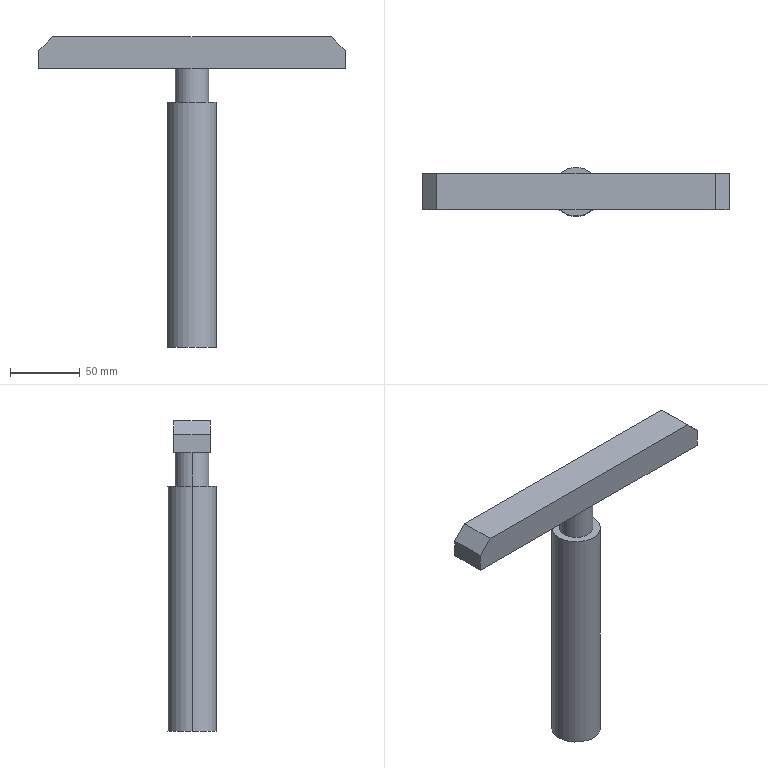Part | SolidWorks | features ICE 2, Chamfer 1, Extrusion 1 | 1 solid | 14 faces | box 220 x 35 x 223 mm | volume 309149 mm3 | plane 10 | cylinder 4 | commonest cylinder face diameters 24 x2 35 x2
STEP:
#1=CARTESIAN_POINT('',(12.,0.,176.));
#2=VERTEX_POINT('',#1);
#3=CARTESIAN_POINT('',(-12.,0.,176.));
#4=VERTEX_POINT('',#3);
#5=CARTESIAN_POINT('',(0.,0.,176.));
#6=DIRECTION('',(0.,0.,1.));
#7=DIRECTION('',(1.,0.,0.));
#8=AXIS2_PLACEMENT_3D('',#5,#6,#7);
#9=CIRCLE('',#8,12.);
#10=EDGE_CURVE('',#2,#4,#9,.T.);
#11=ORIENTED_EDGE('',*,*,#10,.T.);
#12=CARTESIAN_POINT('',(-12.,0.,200.));
#13=VERTEX_POINT('',#12);
#14=CARTESIAN_POINT('',(-12.,0.,176.));
#15=DIRECTION('',(0.,0.,1.));
#16=VECTOR('',#15,1000.);
#17=LINE('',#14,#16);
#18=EDGE_CURVE('',#4,#13,#17,.T.);
#19=ORIENTED_EDGE('',*,*,#18,.T.);
#20=CARTESIAN_POINT('',(12.,0.,200.));
#21=VERTEX_POINT('',#20);
#22=CARTESIAN_POINT('',(0.,0.,200.));
#23=DIRECTION('',(0.,0.,1.));
#24=DIRECTION('',(1.,0.,0.));
#25=AXIS2_PLACEMENT_3D('',#22,#23,#24);
#26=CIRCLE('',#25,12.);
#27=EDGE_CURVE('',#21,#13,#26,.T.);
#28=ORIENTED_EDGE('',*,*,#27,.F.);
#29=CARTESIAN_POINT('',(12.,0.,176.));
#30=DIRECTION('',(0.,0.,1.));
#31=VECTOR('',#30,1000.);
#32=LINE('',#29,#31);
#33=EDGE_CURVE('',#2,#21,#32,.T.);
#34=ORIENTED_EDGE('',*,*,#33,.F.);
#35=EDGE_LOOP('',(#11,#19,#28,#34));
#36=FACE_OUTER_BOUND('',#35,.T.);
#37=CARTESIAN_POINT('',(0.,0.,176.));
#38=DIRECTION('',(0.,0.,1.));
#39=DIRECTION('',(1.,0.,0.));
#40=AXIS2_PLACEMENT_3D('',#37,#38,#39);
#41=CYLINDRICAL_SURFACE('',#40,12.);
#42=ADVANCED_FACE('',(#36),#41,.T.);
#43=CARTESIAN_POINT('',(17.5,0.,176.));
#44=VERTEX_POINT('',#43);
#45=CARTESIAN_POINT('',(-17.5,0.,176.));
#46=VERTEX_POINT('',#45);
#47=CARTESIAN_POINT('',(0.,0.,176.));
#48=DIRECTION('',(0.,0.,1.));
#49=DIRECTION('',(1.,0.,0.));
#50=AXIS2_PLACEMENT_3D('',#47,#48,#49);
#51=CIRCLE('',#50,17.5);
#52=EDGE_CURVE('',#44,#46,#51,.T.);
#53=ORIENTED_EDGE('',*,*,#52,.F.);
#54=CARTESIAN_POINT('',(17.5,0.,0.));
#55=VERTEX_POINT('',#54);
#56=CARTESIAN_POINT('',(17.5,0.,200.));
#57=DIRECTION('',(0.,0.,-1.));
#58=VECTOR('',#57,1000.);
#59=LINE('',#56,#58);
#60=EDGE_CURVE('',#44,#55,#59,.T.);
#61=ORIENTED_EDGE('',*,*,#60,.T.);
#62=CARTESIAN_POINT('',(-17.5,0.,0.));
#63=VERTEX_POINT('',#62);
#64=CARTESIAN_POINT('',(0.,0.,0.));
#65=DIRECTION('',(0.,0.,1.));
#66=DIRECTION('',(1.,0.,0.));
#67=AXIS2_PLACEMENT_3D('',#64,#65,#66);
#68=CIRCLE('',#67,17.5);
#69=EDGE_CURVE('',#55,#63,#68,.T.);
#70=ORIENTED_EDGE('',*,*,#69,.T.);
#71=CARTESIAN_POINT('',(-17.5,0.,200.));
#72=DIRECTION('',(0.,0.,-1.));
#73=VECTOR('',#72,1000.);
#74=LINE('',#71,#73);
#75=EDGE_CURVE('',#46,#63,#74,.T.);
#76=ORIENTED_EDGE('',*,*,#75,.F.);
#77=EDGE_LOOP('',(#53,#61,#70,#76));
#78=FACE_OUTER_BOUND('',#77,.T.);
#79=CARTESIAN_POINT('',(0.,0.,200.));
#80=DIRECTION('',(0.,0.,-1.));
#81=DIRECTION('',(-1.,0.,0.));
#82=AXIS2_PLACEMENT_3D('',#79,#80,#81);
#83=CYLINDRICAL_SURFACE('',#82,17.5);
#84=ADVANCED_FACE('',(#78),#83,.T.);
#85=ORIENTED_EDGE('',*,*,#60,.F.);
#86=CARTESIAN_POINT('',(0.,0.,176.));
#87=DIRECTION('',(0.,0.,1.));
#88=DIRECTION('',(1.,0.,0.));
#89=AXIS2_PLACEMENT_3D('',#86,#87,#88);
#90=CIRCLE('',#89,17.5);
#91=EDGE_CURVE('',#46,#44,#90,.T.);
#92=ORIENTED_EDGE('',*,*,#91,.F.);
#93=ORIENTED_EDGE('',*,*,#75,.T.);
#94=CARTESIAN_POINT('',(0.,0.,0.));
#95=DIRECTION('',(0.,0.,1.));
#96=DIRECTION('',(1.,0.,0.));
#97=AXIS2_PLACEMENT_3D('',#94,#95,#96);
#98=CIRCLE('',#97,17.5);
#99=EDGE_CURVE('',#63,#55,#98,.T.);
#100=ORIENTED_EDGE('',*,*,#99,.T.);
#101=EDGE_LOOP('',(#85,#92,#93,#100));
#102=FACE_OUTER_BOUND('',#101,.T.);
#103=CARTESIAN_POINT('',(0.,0.,200.));
#104=DIRECTION('',(0.,0.,-1.));
#105=DIRECTION('',(-1.,0.,0.));
#106=AXIS2_PLACEMENT_3D('',#103,#104,#105);
#107=CYLINDRICAL_SURFACE('',#106,17.5);
#108=ADVANCED_FACE('',(#102),#107,.T.);
#109=ORIENTED_EDGE('',*,*,#99,.F.);
#110=ORIENTED_EDGE('',*,*,#69,.F.);
#111=EDGE_LOOP('',(#109,#110));
#112=FACE_OUTER_BOUND('',#111,.T.);
#113=CARTESIAN_POINT('',(0.,0.,0.));
#114=DIRECTION('',(0.,0.,1.));
#115=DIRECTION('',(1.,0.,0.));
#116=AXIS2_PLACEMENT_3D('',#113,#114,#115);
#117=PLANE('',#116);
#118=ADVANCED_FACE('',(#112),#117,.F.);
#119=ORIENTED_EDGE('',*,*,#10,.F.);
#120=CARTESIAN_POINT('',(0.,0.,176.));
#121=DIRECTION('',(0.,0.,1.));
#122=DIRECTION('',(1.,0.,0.));
#123=AXIS2_PLACEMENT_3D('',#120,#121,#122);
#124=CIRCLE('',#123,12.);
#125=EDGE_CURVE('',#4,#2,#124,.T.);
#126=ORIENTED_EDGE('',*,*,#125,.F.);
#127=EDGE_LOOP('',(#119,#126));
#128=FACE_BOUND('',#127,.T.);
#129=ORIENTED_EDGE('',*,*,#91,.T.);
#130=ORIENTED_EDGE('',*,*,#52,.T.);
#131=EDGE_LOOP('',(#129,#130));
#132=FACE_OUTER_BOUND('',#131,.T.);
#133=CARTESIAN_POINT('',(0.,0.,176.));
#134=DIRECTION('',(0.,0.,1.));
#135=DIRECTION('',(1.,0.,0.));
#136=AXIS2_PLACEMENT_3D('',#133,#134,#135);
#137=PLANE('',#136);
#138=ADVANCED_FACE('',(#128,#132),#137,.T.);
#139=ORIENTED_EDGE('',*,*,#18,.F.);
#140=ORIENTED_EDGE('',*,*,#125,.T.);
#141=ORIENTED_EDGE('',*,*,#33,.T.);
#142=CARTESIAN_POINT('',(0.,0.,200.));
#143=DIRECTION('',(0.,0.,1.));
#144=DIRECTION('',(1.,0.,0.));
#145=AXIS2_PLACEMENT_3D('',#142,#143,#144);
#146=CIRCLE('',#145,12.);
#147=EDGE_CURVE('',#13,#21,#146,.T.);
#148=ORIENTED_EDGE('',*,*,#147,.F.);
#149=EDGE_LOOP('',(#139,#140,#141,#148));
#150=FACE_OUTER_BOUND('',#149,.T.);
#151=CARTESIAN_POINT('',(0.,0.,176.));
#152=DIRECTION('',(0.,0.,1.));
#153=DIRECTION('',(1.,0.,0.));
#154=AXIS2_PLACEMENT_3D('',#151,#152,#153);
#155=CYLINDRICAL_SURFACE('',#154,12.);
#156=ADVANCED_FACE('',(#150),#155,.T.);
#157=CARTESIAN_POINT('',(-110.,-13.,213.));
#158=VERTEX_POINT('',#157);
#159=CARTESIAN_POINT('',(-110.,-13.,200.));
#160=VERTEX_POINT('',#159);
#161=CARTESIAN_POINT('',(-110.,-13.,223.));
#162=DIRECTION('',(0.,0.,-1.));
#163=VECTOR('',#162,1000.);
#164=LINE('',#161,#163);
#165=EDGE_CURVE('',#158,#160,#164,.T.);
#166=ORIENTED_EDGE('',*,*,#165,.F.);
#167=CARTESIAN_POINT('',(-110.,13.,213.));
#168=VERTEX_POINT('',#167);
#169=CARTESIAN_POINT('',(-110.,13.,213.));
#170=DIRECTION('',(0.,1.,0.));
#171=VECTOR('',#170,1000.);
#172=LINE('',#169,#171);
#173=EDGE_CURVE('',#158,#168,#172,.T.);
#174=ORIENTED_EDGE('',*,*,#173,.T.);
#175=CARTESIAN_POINT('',(-110.,13.,200.));
#176=VERTEX_POINT('',#175);
#177=CARTESIAN_POINT('',(-110.,13.,223.));
#178=DIRECTION('',(0.,0.,-1.));
#179=VECTOR('',#178,1000.);
#180=LINE('',#177,#179);
#181=EDGE_CURVE('',#168,#176,#180,.T.);
#182=ORIENTED_EDGE('',*,*,#181,.T.);
#183=CARTESIAN_POINT('',(-110.,-13.,200.));
#184=DIRECTION('',(0.,-1.,0.));
#185=VECTOR('',#184,1000.);
#186=LINE('',#183,#185);
#187=EDGE_CURVE('',#176,#160,#186,.T.);
#188=ORIENTED_EDGE('',*,*,#187,.T.);
#189=EDGE_LOOP('',(#166,#174,#182,#188));
#190=FACE_OUTER_BOUND('',#189,.T.);
#191=CARTESIAN_POINT('',(-110.,-13.,223.));
#192=DIRECTION('',(1.,0.,0.));
#193=DIRECTION('',(0.,0.,-1.));
#194=AXIS2_PLACEMENT_3D('',#191,#192,#193);
#195=PLANE('',#194);
#196=ADVANCED_FACE('',(#190),#195,.F.);
#197=CARTESIAN_POINT('',(110.,-13.,213.));
#198=VERTEX_POINT('',#197);
#199=CARTESIAN_POINT('',(110.,-13.,200.));
#200=VERTEX_POINT('',#199);
#201=CARTESIAN_POINT('',(110.,-13.,223.));
#202=DIRECTION('',(0.,0.,-1.));
#203=VECTOR('',#202,1000.);
#204=LINE('',#201,#203);
#205=EDGE_CURVE('',#198,#200,#204,.T.);
#206=ORIENTED_EDGE('',*,*,#205,.F.);
#207=CARTESIAN_POINT('',(100.,-13.,223.));
#208=VERTEX_POINT('',#207);
#209=CARTESIAN_POINT('',(100.,-13.,223.));
#210=DIRECTION('',(-0.7071,0.,0.7071));
#211=VECTOR('',#210,1000.);
#212=LINE('',#209,#211);
#213=EDGE_CURVE('',#198,#208,#212,.T.);
#214=ORIENTED_EDGE('',*,*,#213,.T.);
#215=CARTESIAN_POINT('',(-100.,-13.,223.));
#216=VERTEX_POINT('',#215);
#217=CARTESIAN_POINT('',(110.,-13.,223.));
#218=DIRECTION('',(1.,0.,0.));
#219=VECTOR('',#218,1000.);
#220=LINE('',#217,#219);
#221=EDGE_CURVE('',#216,#208,#220,.T.);
#222=ORIENTED_EDGE('',*,*,#221,.F.);
#223=CARTESIAN_POINT('',(-100.,-13.,223.));
#224=DIRECTION('',(-0.7071,0.,-0.7071));
#225=VECTOR('',#224,1000.);
#226=LINE('',#223,#225);
#227=EDGE_CURVE('',#216,#158,#226,.T.);
#228=ORIENTED_EDGE('',*,*,#227,.T.);
#229=ORIENTED_EDGE('',*,*,#165,.T.);
#230=CARTESIAN_POINT('',(110.,-13.,200.));
#231=DIRECTION('',(1.,0.,0.));
#232=VECTOR('',#231,1000.);
#233=LINE('',#230,#232);
#234=EDGE_CURVE('',#160,#200,#233,.T.);
#235=ORIENTED_EDGE('',*,*,#234,.T.);
#236=EDGE_LOOP('',(#206,#214,#222,#228,#229,#235));
#237=FACE_OUTER_BOUND('',#236,.T.);
#238=CARTESIAN_POINT('',(110.,-13.,223.));
#239=DIRECTION('',(0.,1.,0.));
#240=DIRECTION('',(-1.,0.,0.));
#241=AXIS2_PLACEMENT_3D('',#238,#239,#240);
#242=PLANE('',#241);
#243=ADVANCED_FACE('',(#237),#242,.F.);
#244=CARTESIAN_POINT('',(110.,13.,213.));
#245=VERTEX_POINT('',#244);
#246=CARTESIAN_POINT('',(110.,13.,200.));
#247=VERTEX_POINT('',#246);
#248=CARTESIAN_POINT('',(110.,13.,223.));
#249=DIRECTION('',(0.,0.,-1.));
#250=VECTOR('',#249,1000.);
#251=LINE('',#248,#250);
#252=EDGE_CURVE('',#245,#247,#251,.T.);
#253=ORIENTED_EDGE('',*,*,#252,.F.);
#254=CARTESIAN_POINT('',(110.,-13.,213.));
#255=DIRECTION('',(0.,-1.,0.));
#256=VECTOR('',#255,1000.);
#257=LINE('',#254,#256);
#258=EDGE_CURVE('',#245,#198,#257,.T.);
#259=ORIENTED_EDGE('',*,*,#258,.T.);
#260=ORIENTED_EDGE('',*,*,#205,.T.);
#261=CARTESIAN_POINT('',(110.,-13.,200.));
#262=DIRECTION('',(0.,1.,0.));
#263=VECTOR('',#262,1000.);
#264=LINE('',#261,#263);
#265=EDGE_CURVE('',#200,#247,#264,.T.);
#266=ORIENTED_EDGE('',*,*,#265,.T.);
#267=EDGE_LOOP('',(#253,#259,#260,#266));
#268=FACE_OUTER_BOUND('',#267,.T.);
#269=CARTESIAN_POINT('',(110.,-13.,223.));
#270=DIRECTION('',(-1.,0.,0.));
#271=DIRECTION('',(0.,0.,1.));
#272=AXIS2_PLACEMENT_3D('',#269,#270,#271);
#273=PLANE('',#272);
#274=ADVANCED_FACE('',(#268),#273,.F.);
#275=CARTESIAN_POINT('',(100.,13.,223.));
#276=VERTEX_POINT('',#275);
#277=CARTESIAN_POINT('',(-100.,13.,223.));
#278=VERTEX_POINT('',#277);
#279=CARTESIAN_POINT('',(110.,13.,223.));
#280=DIRECTION('',(-1.,0.,0.));
#281=VECTOR('',#280,1000.);
#282=LINE('',#279,#281);
#283=EDGE_CURVE('',#276,#278,#282,.T.);
#284=ORIENTED_EDGE('',*,*,#283,.F.);
#285=CARTESIAN_POINT('',(100.,13.,223.));
#286=DIRECTION('',(0.7071,0.,-0.7071));
#287=VECTOR('',#286,1000.);
#288=LINE('',#285,#287);
#289=EDGE_CURVE('',#276,#245,#288,.T.);
#290=ORIENTED_EDGE('',*,*,#289,.T.);
#291=ORIENTED_EDGE('',*,*,#252,.T.);
#292=CARTESIAN_POINT('',(110.,13.,200.));
#293=DIRECTION('',(-1.,0.,0.));
#294=VECTOR('',#293,1000.);
#295=LINE('',#292,#294);
#296=EDGE_CURVE('',#247,#176,#295,.T.);
#297=ORIENTED_EDGE('',*,*,#296,.T.);
#298=ORIENTED_EDGE('',*,*,#181,.F.);
#299=CARTESIAN_POINT('',(-100.,13.,223.));
#300=DIRECTION('',(0.7071,0.,0.7071));
#301=VECTOR('',#300,1000.);
#302=LINE('',#299,#301);
#303=EDGE_CURVE('',#168,#278,#302,.T.);
#304=ORIENTED_EDGE('',*,*,#303,.T.);
#305=EDGE_LOOP('',(#284,#290,#291,#297,#298,#304));
#306=FACE_OUTER_BOUND('',#305,.T.);
#307=CARTESIAN_POINT('',(110.,13.,223.));
#308=DIRECTION('',(0.,-1.,0.));
#309=DIRECTION('',(1.,0.,0.));
#310=AXIS2_PLACEMENT_3D('',#307,#308,#309);
#311=PLANE('',#310);
#312=ADVANCED_FACE('',(#306),#311,.F.);
#313=ORIENTED_EDGE('',*,*,#221,.T.);
#314=CARTESIAN_POINT('',(100.,13.,223.));
#315=DIRECTION('',(0.,1.,0.));
#316=VECTOR('',#315,1000.);
#317=LINE('',#314,#316);
#318=EDGE_CURVE('',#208,#276,#317,.T.);
#319=ORIENTED_EDGE('',*,*,#318,.T.);
#320=ORIENTED_EDGE('',*,*,#283,.T.);
#321=CARTESIAN_POINT('',(-100.,-13.,223.));
#322=DIRECTION('',(0.,-1.,0.));
#323=VECTOR('',#322,1000.);
#324=LINE('',#321,#323);
#325=EDGE_CURVE('',#278,#216,#324,.T.);
#326=ORIENTED_EDGE('',*,*,#325,.T.);
#327=EDGE_LOOP('',(#313,#319,#320,#326));
#328=FACE_OUTER_BOUND('',#327,.T.);
#329=CARTESIAN_POINT('',(0.,0.,223.));
#330=DIRECTION('',(0.,0.,1.));
#331=DIRECTION('',(1.,0.,0.));
#332=AXIS2_PLACEMENT_3D('',#329,#330,#331);
#333=PLANE('',#332);
#334=ADVANCED_FACE('',(#328),#333,.T.);
#335=ORIENTED_EDGE('',*,*,#27,.T.);
#336=ORIENTED_EDGE('',*,*,#147,.T.);
#337=EDGE_LOOP('',(#335,#336));
#338=FACE_BOUND('',#337,.T.);
#339=ORIENTED_EDGE('',*,*,#187,.F.);
#340=ORIENTED_EDGE('',*,*,#296,.F.);
#341=ORIENTED_EDGE('',*,*,#265,.F.);
#342=ORIENTED_EDGE('',*,*,#234,.F.);
#343=EDGE_LOOP('',(#339,#340,#341,#342));
#344=FACE_OUTER_BOUND('',#343,.T.);
#345=CARTESIAN_POINT('',(0.,0.,200.));
#346=DIRECTION('',(0.,0.,1.));
#347=DIRECTION('',(1.,0.,0.));
#348=AXIS2_PLACEMENT_3D('',#345,#346,#347);
#349=PLANE('',#348);
#350=ADVANCED_FACE('',(#338,#344),#349,.F.);
#351=ORIENTED_EDGE('',*,*,#213,.F.);
#352=ORIENTED_EDGE('',*,*,#258,.F.);
#353=ORIENTED_EDGE('',*,*,#289,.F.);
#354=ORIENTED_EDGE('',*,*,#318,.F.);
#355=EDGE_LOOP('',(#351,#352,#353,#354));
#356=FACE_OUTER_BOUND('',#355,.T.);
#357=CARTESIAN_POINT('',(100.,0.,223.));
#358=DIRECTION('',(0.7071,0.,0.7071));
#359=DIRECTION('',(0.,-1.,0.));
#360=AXIS2_PLACEMENT_3D('',#357,#358,#359);
#361=PLANE('',#360);
#362=ADVANCED_FACE('',(#356),#361,.T.);
#363=ORIENTED_EDGE('',*,*,#303,.F.);
#364=ORIENTED_EDGE('',*,*,#173,.F.);
#365=ORIENTED_EDGE('',*,*,#227,.F.);
#366=ORIENTED_EDGE('',*,*,#325,.F.);
#367=EDGE_LOOP('',(#363,#364,#365,#366));
#368=FACE_OUTER_BOUND('',#367,.T.);
#369=CARTESIAN_POINT('',(-100.,0.,223.));
#370=DIRECTION('',(-0.7071,0.,0.7071));
#371=DIRECTION('',(0.,1.,0.));
#372=AXIS2_PLACEMENT_3D('',#369,#370,#371);
#373=PLANE('',#372);
#374=ADVANCED_FACE('',(#368),#373,.T.);
#375=CLOSED_SHELL('',(#42,#84,#108,#118,#138,#156,#196,#243,#274,#312,#334,#350,#362,#374));
#376=MANIFOLD_SOLID_BREP('',#375);
#377=CARTESIAN_POINT('',(0.,0.,0.));
#378=DIRECTION('',(0.,0.,1.));
#379=DIRECTION('',(1.,0.,0.));
#380=AXIS2_PLACEMENT_3D('',#377,#378,#379);
#381=(LENGTH_UNIT()NAMED_UNIT(*)SI_UNIT(.MILLI.,.METRE.));
#382=UNCERTAINTY_MEASURE_WITH_UNIT(LENGTH_MEASURE(0.00001),#381,'','');
#383=(NAMED_UNIT(*)PLANE_ANGLE_UNIT()SI_UNIT($,.RADIAN.));
#384=(NAMED_UNIT(*)SI_UNIT($,.STERADIAN.)SOLID_ANGLE_UNIT());
#385=(GEOMETRIC_REPRESENTATION_CONTEXT(3)GLOBAL_UNCERTAINTY_ASSIGNED_CONTEXT((#382))GLOBAL_UNIT_ASSIGNED_CONTEXT((#381,#383,#384))REPRESENTATION_CONTEXT('',''));
#386=ADVANCED_BREP_SHAPE_REPRESENTATION('',(#376,#380),#385);